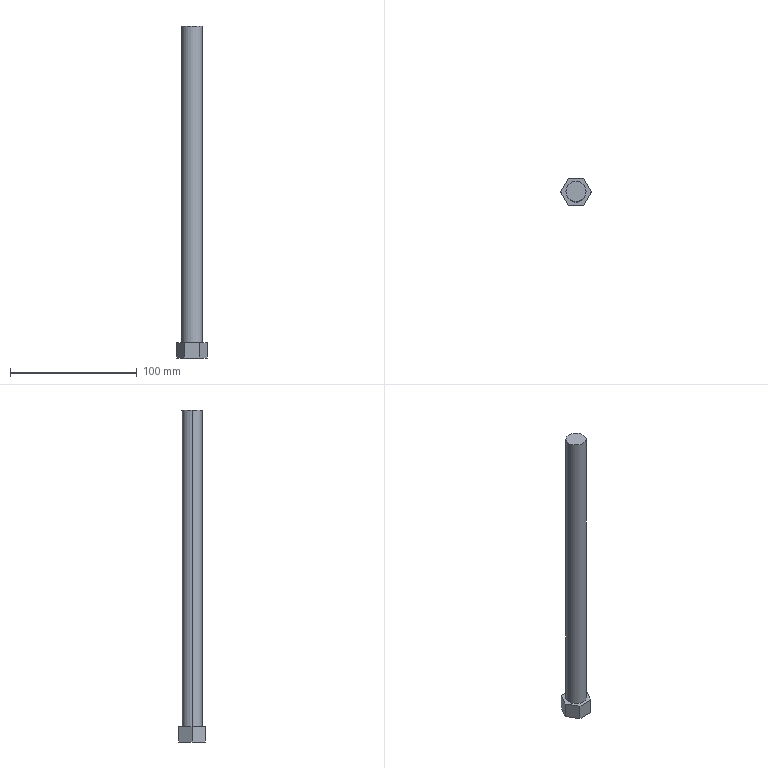Part | SolidWorks | features Extrusion 1, ICE 1 | 1 solid | 11 faces | box 24 x 20.785 x 262 mm | volume 54755 mm3 | plane 9 | cylinder 2 | commonest cylinder face diameters 16 x2
STEP:
#1=CARTESIAN_POINT('',(8.,0.,250.));
#2=VERTEX_POINT('',#1);
#3=CARTESIAN_POINT('',(-8.,0.,250.));
#4=VERTEX_POINT('',#3);
#5=CARTESIAN_POINT('',(0.,0.,250.));
#6=DIRECTION('',(0.,0.,1.));
#7=DIRECTION('',(1.,0.,0.));
#8=AXIS2_PLACEMENT_3D('',#5,#6,#7);
#9=CIRCLE('',#8,8.);
#10=EDGE_CURVE('',#2,#4,#9,.T.);
#11=ORIENTED_EDGE('',*,*,#10,.F.);
#12=CARTESIAN_POINT('',(8.,0.,0.));
#13=VERTEX_POINT('',#12);
#14=CARTESIAN_POINT('',(8.,0.,250.));
#15=DIRECTION('',(0.,0.,-1.));
#16=VECTOR('',#15,1000.);
#17=LINE('',#14,#16);
#18=EDGE_CURVE('',#2,#13,#17,.T.);
#19=ORIENTED_EDGE('',*,*,#18,.T.);
#20=CARTESIAN_POINT('',(-8.,0.,0.));
#21=VERTEX_POINT('',#20);
#22=CARTESIAN_POINT('',(0.,0.,0.));
#23=DIRECTION('',(0.,0.,1.));
#24=DIRECTION('',(1.,0.,0.));
#25=AXIS2_PLACEMENT_3D('',#22,#23,#24);
#26=CIRCLE('',#25,8.);
#27=EDGE_CURVE('',#13,#21,#26,.T.);
#28=ORIENTED_EDGE('',*,*,#27,.T.);
#29=CARTESIAN_POINT('',(-8.,0.,250.));
#30=DIRECTION('',(0.,0.,-1.));
#31=VECTOR('',#30,1000.);
#32=LINE('',#29,#31);
#33=EDGE_CURVE('',#4,#21,#32,.T.);
#34=ORIENTED_EDGE('',*,*,#33,.F.);
#35=EDGE_LOOP('',(#11,#19,#28,#34));
#36=FACE_OUTER_BOUND('',#35,.T.);
#37=CARTESIAN_POINT('',(0.,0.,250.));
#38=DIRECTION('',(0.,0.,-1.));
#39=DIRECTION('',(-1.,0.,0.));
#40=AXIS2_PLACEMENT_3D('',#37,#38,#39);
#41=CYLINDRICAL_SURFACE('',#40,8.);
#42=ADVANCED_FACE('',(#36),#41,.T.);
#43=ORIENTED_EDGE('',*,*,#18,.F.);
#44=CARTESIAN_POINT('',(0.,0.,250.));
#45=DIRECTION('',(0.,0.,1.));
#46=DIRECTION('',(1.,0.,0.));
#47=AXIS2_PLACEMENT_3D('',#44,#45,#46);
#48=CIRCLE('',#47,8.);
#49=EDGE_CURVE('',#4,#2,#48,.T.);
#50=ORIENTED_EDGE('',*,*,#49,.F.);
#51=ORIENTED_EDGE('',*,*,#33,.T.);
#52=CARTESIAN_POINT('',(0.,0.,0.));
#53=DIRECTION('',(0.,0.,1.));
#54=DIRECTION('',(1.,0.,0.));
#55=AXIS2_PLACEMENT_3D('',#52,#53,#54);
#56=CIRCLE('',#55,8.);
#57=EDGE_CURVE('',#21,#13,#56,.T.);
#58=ORIENTED_EDGE('',*,*,#57,.T.);
#59=EDGE_LOOP('',(#43,#50,#51,#58));
#60=FACE_OUTER_BOUND('',#59,.T.);
#61=CARTESIAN_POINT('',(0.,0.,250.));
#62=DIRECTION('',(0.,0.,-1.));
#63=DIRECTION('',(-1.,0.,0.));
#64=AXIS2_PLACEMENT_3D('',#61,#62,#63);
#65=CYLINDRICAL_SURFACE('',#64,8.);
#66=ADVANCED_FACE('',(#60),#65,.T.);
#67=ORIENTED_EDGE('',*,*,#49,.T.);
#68=ORIENTED_EDGE('',*,*,#10,.T.);
#69=EDGE_LOOP('',(#67,#68));
#70=FACE_OUTER_BOUND('',#69,.T.);
#71=CARTESIAN_POINT('',(0.,0.,250.));
#72=DIRECTION('',(0.,0.,1.));
#73=DIRECTION('',(1.,0.,0.));
#74=AXIS2_PLACEMENT_3D('',#71,#72,#73);
#75=PLANE('',#74);
#76=ADVANCED_FACE('',(#70),#75,.T.);
#77=CARTESIAN_POINT('',(6.,-10.392,0.));
#78=VERTEX_POINT('',#77);
#79=CARTESIAN_POINT('',(12.,0.,0.));
#80=VERTEX_POINT('',#79);
#81=CARTESIAN_POINT('',(6.,-10.392,0.));
#82=DIRECTION('',(0.5,0.866,0.));
#83=VECTOR('',#82,1000.);
#84=LINE('',#81,#83);
#85=EDGE_CURVE('',#78,#80,#84,.T.);
#86=ORIENTED_EDGE('',*,*,#85,.F.);
#87=CARTESIAN_POINT('',(6.,-10.392,-12.));
#88=VERTEX_POINT('',#87);
#89=CARTESIAN_POINT('',(6.,-10.392,-12.));
#90=DIRECTION('',(0.,0.,1.));
#91=VECTOR('',#90,1000.);
#92=LINE('',#89,#91);
#93=EDGE_CURVE('',#88,#78,#92,.T.);
#94=ORIENTED_EDGE('',*,*,#93,.F.);
#95=CARTESIAN_POINT('',(12.,0.,-12.));
#96=VERTEX_POINT('',#95);
#97=CARTESIAN_POINT('',(6.,-10.392,-12.));
#98=DIRECTION('',(0.5,0.866,0.));
#99=VECTOR('',#98,1000.);
#100=LINE('',#97,#99);
#101=EDGE_CURVE('',#88,#96,#100,.T.);
#102=ORIENTED_EDGE('',*,*,#101,.T.);
#103=CARTESIAN_POINT('',(12.,0.,-12.));
#104=DIRECTION('',(0.,0.,1.));
#105=VECTOR('',#104,1000.);
#106=LINE('',#103,#105);
#107=EDGE_CURVE('',#96,#80,#106,.T.);
#108=ORIENTED_EDGE('',*,*,#107,.T.);
#109=EDGE_LOOP('',(#86,#94,#102,#108));
#110=FACE_OUTER_BOUND('',#109,.T.);
#111=CARTESIAN_POINT('',(6.,-10.392,-12.));
#112=DIRECTION('',(0.866,-0.5,0.));
#113=DIRECTION('',(0.5,0.866,0.));
#114=AXIS2_PLACEMENT_3D('',#111,#112,#113);
#115=PLANE('',#114);
#116=ADVANCED_FACE('',(#110),#115,.T.);
#117=CARTESIAN_POINT('',(-6.,-10.392,0.));
#118=VERTEX_POINT('',#117);
#119=CARTESIAN_POINT('',(-6.,-10.392,0.));
#120=DIRECTION('',(1.,0.,0.));
#121=VECTOR('',#120,1000.);
#122=LINE('',#119,#121);
#123=EDGE_CURVE('',#118,#78,#122,.T.);
#124=ORIENTED_EDGE('',*,*,#123,.F.);
#125=CARTESIAN_POINT('',(-6.,-10.392,-12.));
#126=VERTEX_POINT('',#125);
#127=CARTESIAN_POINT('',(-6.,-10.392,-12.));
#128=DIRECTION('',(0.,0.,1.));
#129=VECTOR('',#128,1000.);
#130=LINE('',#127,#129);
#131=EDGE_CURVE('',#126,#118,#130,.T.);
#132=ORIENTED_EDGE('',*,*,#131,.F.);
#133=CARTESIAN_POINT('',(-6.,-10.392,-12.));
#134=DIRECTION('',(1.,0.,0.));
#135=VECTOR('',#134,1000.);
#136=LINE('',#133,#135);
#137=EDGE_CURVE('',#126,#88,#136,.T.);
#138=ORIENTED_EDGE('',*,*,#137,.T.);
#139=ORIENTED_EDGE('',*,*,#93,.T.);
#140=EDGE_LOOP('',(#124,#132,#138,#139));
#141=FACE_OUTER_BOUND('',#140,.T.);
#142=CARTESIAN_POINT('',(-6.,-10.392,-12.));
#143=DIRECTION('',(0.,-1.,0.));
#144=DIRECTION('',(1.,0.,0.));
#145=AXIS2_PLACEMENT_3D('',#142,#143,#144);
#146=PLANE('',#145);
#147=ADVANCED_FACE('',(#141),#146,.T.);
#148=CARTESIAN_POINT('',(-12.,0.,0.));
#149=VERTEX_POINT('',#148);
#150=CARTESIAN_POINT('',(-12.,0.,0.));
#151=DIRECTION('',(0.5,-0.866,0.));
#152=VECTOR('',#151,1000.);
#153=LINE('',#150,#152);
#154=EDGE_CURVE('',#149,#118,#153,.T.);
#155=ORIENTED_EDGE('',*,*,#154,.F.);
#156=CARTESIAN_POINT('',(-12.,0.,-12.));
#157=VERTEX_POINT('',#156);
#158=CARTESIAN_POINT('',(-12.,0.,-12.));
#159=DIRECTION('',(0.,0.,1.));
#160=VECTOR('',#159,1000.);
#161=LINE('',#158,#160);
#162=EDGE_CURVE('',#157,#149,#161,.T.);
#163=ORIENTED_EDGE('',*,*,#162,.F.);
#164=CARTESIAN_POINT('',(-12.,0.,-12.));
#165=DIRECTION('',(0.5,-0.866,0.));
#166=VECTOR('',#165,1000.);
#167=LINE('',#164,#166);
#168=EDGE_CURVE('',#157,#126,#167,.T.);
#169=ORIENTED_EDGE('',*,*,#168,.T.);
#170=ORIENTED_EDGE('',*,*,#131,.T.);
#171=EDGE_LOOP('',(#155,#163,#169,#170));
#172=FACE_OUTER_BOUND('',#171,.T.);
#173=CARTESIAN_POINT('',(-12.,0.,-12.));
#174=DIRECTION('',(-0.866,-0.5,0.));
#175=DIRECTION('',(0.5,-0.866,0.));
#176=AXIS2_PLACEMENT_3D('',#173,#174,#175);
#177=PLANE('',#176);
#178=ADVANCED_FACE('',(#172),#177,.T.);
#179=CARTESIAN_POINT('',(-6.,10.392,0.));
#180=VERTEX_POINT('',#179);
#181=CARTESIAN_POINT('',(-6.,10.392,0.));
#182=DIRECTION('',(-0.5,-0.866,0.));
#183=VECTOR('',#182,1000.);
#184=LINE('',#181,#183);
#185=EDGE_CURVE('',#180,#149,#184,.T.);
#186=ORIENTED_EDGE('',*,*,#185,.F.);
#187=CARTESIAN_POINT('',(-6.,10.392,-12.));
#188=VERTEX_POINT('',#187);
#189=CARTESIAN_POINT('',(-6.,10.392,-12.));
#190=DIRECTION('',(0.,0.,1.));
#191=VECTOR('',#190,1000.);
#192=LINE('',#189,#191);
#193=EDGE_CURVE('',#188,#180,#192,.T.);
#194=ORIENTED_EDGE('',*,*,#193,.F.);
#195=CARTESIAN_POINT('',(-6.,10.392,-12.));
#196=DIRECTION('',(-0.5,-0.866,0.));
#197=VECTOR('',#196,1000.);
#198=LINE('',#195,#197);
#199=EDGE_CURVE('',#188,#157,#198,.T.);
#200=ORIENTED_EDGE('',*,*,#199,.T.);
#201=ORIENTED_EDGE('',*,*,#162,.T.);
#202=EDGE_LOOP('',(#186,#194,#200,#201));
#203=FACE_OUTER_BOUND('',#202,.T.);
#204=CARTESIAN_POINT('',(-6.,10.392,-12.));
#205=DIRECTION('',(-0.866,0.5,0.));
#206=DIRECTION('',(-0.5,-0.866,0.));
#207=AXIS2_PLACEMENT_3D('',#204,#205,#206);
#208=PLANE('',#207);
#209=ADVANCED_FACE('',(#203),#208,.T.);
#210=CARTESIAN_POINT('',(6.,10.392,0.));
#211=VERTEX_POINT('',#210);
#212=CARTESIAN_POINT('',(6.,10.392,0.));
#213=DIRECTION('',(-1.,0.,0.));
#214=VECTOR('',#213,1000.);
#215=LINE('',#212,#214);
#216=EDGE_CURVE('',#211,#180,#215,.T.);
#217=ORIENTED_EDGE('',*,*,#216,.F.);
#218=CARTESIAN_POINT('',(6.,10.392,-12.));
#219=VERTEX_POINT('',#218);
#220=CARTESIAN_POINT('',(6.,10.392,-12.));
#221=DIRECTION('',(0.,0.,1.));
#222=VECTOR('',#221,1000.);
#223=LINE('',#220,#222);
#224=EDGE_CURVE('',#219,#211,#223,.T.);
#225=ORIENTED_EDGE('',*,*,#224,.F.);
#226=CARTESIAN_POINT('',(6.,10.392,-12.));
#227=DIRECTION('',(-1.,0.,0.));
#228=VECTOR('',#227,1000.);
#229=LINE('',#226,#228);
#230=EDGE_CURVE('',#219,#188,#229,.T.);
#231=ORIENTED_EDGE('',*,*,#230,.T.);
#232=ORIENTED_EDGE('',*,*,#193,.T.);
#233=EDGE_LOOP('',(#217,#225,#231,#232));
#234=FACE_OUTER_BOUND('',#233,.T.);
#235=CARTESIAN_POINT('',(6.,10.392,-12.));
#236=DIRECTION('',(0.,1.,0.));
#237=DIRECTION('',(0.,0.,1.));
#238=AXIS2_PLACEMENT_3D('',#235,#236,#237);
#239=PLANE('',#238);
#240=ADVANCED_FACE('',(#234),#239,.T.);
#241=CARTESIAN_POINT('',(12.,0.,0.));
#242=DIRECTION('',(-0.5,0.866,0.));
#243=VECTOR('',#242,1000.);
#244=LINE('',#241,#243);
#245=EDGE_CURVE('',#80,#211,#244,.T.);
#246=ORIENTED_EDGE('',*,*,#245,.F.);
#247=ORIENTED_EDGE('',*,*,#107,.F.);
#248=CARTESIAN_POINT('',(12.,0.,-12.));
#249=DIRECTION('',(-0.5,0.866,0.));
#250=VECTOR('',#249,1000.);
#251=LINE('',#248,#250);
#252=EDGE_CURVE('',#96,#219,#251,.T.);
#253=ORIENTED_EDGE('',*,*,#252,.T.);
#254=ORIENTED_EDGE('',*,*,#224,.T.);
#255=EDGE_LOOP('',(#246,#247,#253,#254));
#256=FACE_OUTER_BOUND('',#255,.T.);
#257=CARTESIAN_POINT('',(12.,0.,-12.));
#258=DIRECTION('',(0.866,0.5,0.));
#259=DIRECTION('',(-0.5,0.866,0.));
#260=AXIS2_PLACEMENT_3D('',#257,#258,#259);
#261=PLANE('',#260);
#262=ADVANCED_FACE('',(#256),#261,.T.);
#263=ORIENTED_EDGE('',*,*,#101,.F.);
#264=ORIENTED_EDGE('',*,*,#137,.F.);
#265=ORIENTED_EDGE('',*,*,#168,.F.);
#266=ORIENTED_EDGE('',*,*,#199,.F.);
#267=ORIENTED_EDGE('',*,*,#230,.F.);
#268=ORIENTED_EDGE('',*,*,#252,.F.);
#269=EDGE_LOOP('',(#263,#264,#265,#266,#267,#268));
#270=FACE_OUTER_BOUND('',#269,.T.);
#271=CARTESIAN_POINT('',(0.,0.,-12.));
#272=DIRECTION('',(0.,0.,1.));
#273=DIRECTION('',(1.,0.,0.));
#274=AXIS2_PLACEMENT_3D('',#271,#272,#273);
#275=PLANE('',#274);
#276=ADVANCED_FACE('',(#270),#275,.F.);
#277=ORIENTED_EDGE('',*,*,#57,.F.);
#278=ORIENTED_EDGE('',*,*,#27,.F.);
#279=EDGE_LOOP('',(#277,#278));
#280=FACE_BOUND('',#279,.T.);
#281=ORIENTED_EDGE('',*,*,#85,.T.);
#282=ORIENTED_EDGE('',*,*,#245,.T.);
#283=ORIENTED_EDGE('',*,*,#216,.T.);
#284=ORIENTED_EDGE('',*,*,#185,.T.);
#285=ORIENTED_EDGE('',*,*,#154,.T.);
#286=ORIENTED_EDGE('',*,*,#123,.T.);
#287=EDGE_LOOP('',(#281,#282,#283,#284,#285,#286));
#288=FACE_OUTER_BOUND('',#287,.T.);
#289=CARTESIAN_POINT('',(0.,0.,0.));
#290=DIRECTION('',(0.,0.,1.));
#291=DIRECTION('',(1.,0.,0.));
#292=AXIS2_PLACEMENT_3D('',#289,#290,#291);
#293=PLANE('',#292);
#294=ADVANCED_FACE('',(#280,#288),#293,.T.);
#295=CLOSED_SHELL('',(#42,#66,#76,#116,#147,#178,#209,#240,#262,#276,#294));
#296=MANIFOLD_SOLID_BREP('',#295);
#297=CARTESIAN_POINT('',(0.,0.,0.));
#298=DIRECTION('',(0.,0.,1.));
#299=DIRECTION('',(1.,0.,0.));
#300=AXIS2_PLACEMENT_3D('',#297,#298,#299);
#301=(LENGTH_UNIT()NAMED_UNIT(*)SI_UNIT(.MILLI.,.METRE.));
#302=UNCERTAINTY_MEASURE_WITH_UNIT(LENGTH_MEASURE(0.00001),#301,'','');
#303=(NAMED_UNIT(*)PLANE_ANGLE_UNIT()SI_UNIT($,.RADIAN.));
#304=(NAMED_UNIT(*)SI_UNIT($,.STERADIAN.)SOLID_ANGLE_UNIT());
#305=(GEOMETRIC_REPRESENTATION_CONTEXT(3)GLOBAL_UNCERTAINTY_ASSIGNED_CONTEXT((#302))GLOBAL_UNIT_ASSIGNED_CONTEXT((#301,#303,#304))REPRESENTATION_CONTEXT('',''));
#306=ADVANCED_BREP_SHAPE_REPRESENTATION('',(#296,#300),#305);